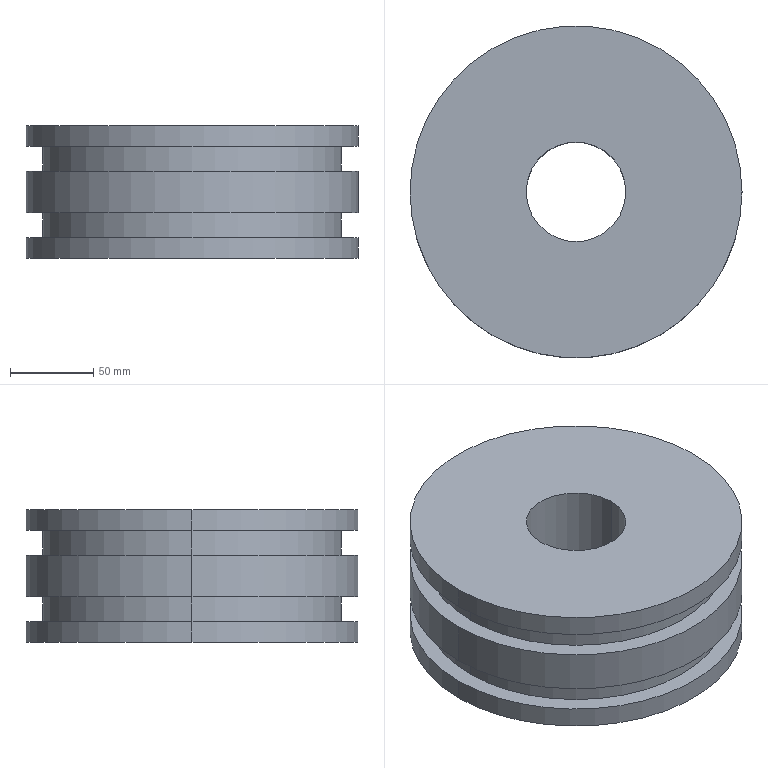Part | SolidWorks | features Extrusion 1, ICE 1, MirrorPattern 1 | 1 solid | 18 faces | box 200 x 200 x 80 mm | volume 2108009 mm3 | cylinder 12 | plane 6 | commonest cylinder face diameters 200 x6 180 x4 60 x2
STEP:
#1=CARTESIAN_POINT('',(90.,0.,-27.5));
#2=VERTEX_POINT('',#1);
#3=CARTESIAN_POINT('',(-90.,0.,-27.5));
#4=VERTEX_POINT('',#3);
#5=CARTESIAN_POINT('',(0.,0.,-27.5));
#6=DIRECTION('',(0.,0.,1.));
#7=DIRECTION('',(1.,0.,0.));
#8=AXIS2_PLACEMENT_3D('',#5,#6,#7);
#9=CIRCLE('',#8,90.);
#10=EDGE_CURVE('',#2,#4,#9,.T.);
#11=ORIENTED_EDGE('',*,*,#10,.T.);
#12=CARTESIAN_POINT('',(-90.,0.,-12.5));
#13=VERTEX_POINT('',#12);
#14=CARTESIAN_POINT('',(-90.,0.,-27.5));
#15=DIRECTION('',(0.,0.,1.));
#16=VECTOR('',#15,1000.);
#17=LINE('',#14,#16);
#18=EDGE_CURVE('',#4,#13,#17,.T.);
#19=ORIENTED_EDGE('',*,*,#18,.T.);
#20=CARTESIAN_POINT('',(90.,0.,-12.5));
#21=VERTEX_POINT('',#20);
#22=CARTESIAN_POINT('',(0.,0.,-12.5));
#23=DIRECTION('',(0.,0.,1.));
#24=DIRECTION('',(1.,0.,0.));
#25=AXIS2_PLACEMENT_3D('',#22,#23,#24);
#26=CIRCLE('',#25,90.);
#27=EDGE_CURVE('',#21,#13,#26,.T.);
#28=ORIENTED_EDGE('',*,*,#27,.F.);
#29=CARTESIAN_POINT('',(90.,0.,-27.5));
#30=DIRECTION('',(0.,0.,1.));
#31=VECTOR('',#30,1000.);
#32=LINE('',#29,#31);
#33=EDGE_CURVE('',#2,#21,#32,.T.);
#34=ORIENTED_EDGE('',*,*,#33,.F.);
#35=EDGE_LOOP('',(#11,#19,#28,#34));
#36=FACE_OUTER_BOUND('',#35,.T.);
#37=CARTESIAN_POINT('',(0.,0.,-27.5));
#38=DIRECTION('',(0.,0.,1.));
#39=DIRECTION('',(1.,0.,0.));
#40=AXIS2_PLACEMENT_3D('',#37,#38,#39);
#41=CYLINDRICAL_SURFACE('',#40,90.);
#42=ADVANCED_FACE('',(#36),#41,.T.);
#43=CARTESIAN_POINT('',(90.,0.,27.5));
#44=VERTEX_POINT('',#43);
#45=CARTESIAN_POINT('',(-90.,0.,27.5));
#46=VERTEX_POINT('',#45);
#47=CARTESIAN_POINT('',(0.,0.,27.5));
#48=DIRECTION('',(0.,0.,1.));
#49=DIRECTION('',(1.,0.,0.));
#50=AXIS2_PLACEMENT_3D('',#47,#48,#49);
#51=CIRCLE('',#50,90.);
#52=EDGE_CURVE('',#44,#46,#51,.T.);
#53=ORIENTED_EDGE('',*,*,#52,.F.);
#54=CARTESIAN_POINT('',(90.,0.,12.5));
#55=VERTEX_POINT('',#54);
#56=CARTESIAN_POINT('',(90.,0.,27.5));
#57=DIRECTION('',(0.,0.,-1.));
#58=VECTOR('',#57,1000.);
#59=LINE('',#56,#58);
#60=EDGE_CURVE('',#44,#55,#59,.T.);
#61=ORIENTED_EDGE('',*,*,#60,.T.);
#62=CARTESIAN_POINT('',(-90.,0.,12.5));
#63=VERTEX_POINT('',#62);
#64=CARTESIAN_POINT('',(0.,0.,12.5));
#65=DIRECTION('',(0.,0.,1.));
#66=DIRECTION('',(1.,0.,0.));
#67=AXIS2_PLACEMENT_3D('',#64,#65,#66);
#68=CIRCLE('',#67,90.);
#69=EDGE_CURVE('',#55,#63,#68,.T.);
#70=ORIENTED_EDGE('',*,*,#69,.T.);
#71=CARTESIAN_POINT('',(-90.,0.,27.5));
#72=DIRECTION('',(0.,0.,-1.));
#73=VECTOR('',#72,1000.);
#74=LINE('',#71,#73);
#75=EDGE_CURVE('',#46,#63,#74,.T.);
#76=ORIENTED_EDGE('',*,*,#75,.F.);
#77=EDGE_LOOP('',(#53,#61,#70,#76));
#78=FACE_OUTER_BOUND('',#77,.T.);
#79=CARTESIAN_POINT('',(0.,0.,27.5));
#80=DIRECTION('',(0.,0.,-1.));
#81=DIRECTION('',(-1.,0.,0.));
#82=AXIS2_PLACEMENT_3D('',#79,#80,#81);
#83=CYLINDRICAL_SURFACE('',#82,90.);
#84=ADVANCED_FACE('',(#78),#83,.T.);
#85=CARTESIAN_POINT('',(-30.,0.,40.));
#86=VERTEX_POINT('',#85);
#87=CARTESIAN_POINT('',(30.,0.,40.));
#88=VERTEX_POINT('',#87);
#89=CARTESIAN_POINT('',(0.,0.,40.));
#90=DIRECTION('',(0.,0.,1.));
#91=DIRECTION('',(1.,0.,0.));
#92=AXIS2_PLACEMENT_3D('',#89,#90,#91);
#93=CIRCLE('',#92,30.);
#94=EDGE_CURVE('',#86,#88,#93,.T.);
#95=ORIENTED_EDGE('',*,*,#94,.T.);
#96=CARTESIAN_POINT('',(30.,0.,-40.));
#97=VERTEX_POINT('',#96);
#98=CARTESIAN_POINT('',(30.,0.,40.));
#99=DIRECTION('',(0.,0.,-1.));
#100=VECTOR('',#99,1000.);
#101=LINE('',#98,#100);
#102=EDGE_CURVE('',#88,#97,#101,.T.);
#103=ORIENTED_EDGE('',*,*,#102,.T.);
#104=CARTESIAN_POINT('',(-30.,0.,-40.));
#105=VERTEX_POINT('',#104);
#106=CARTESIAN_POINT('',(0.,0.,-40.));
#107=DIRECTION('',(0.,0.,1.));
#108=DIRECTION('',(1.,0.,0.));
#109=AXIS2_PLACEMENT_3D('',#106,#107,#108);
#110=CIRCLE('',#109,30.);
#111=EDGE_CURVE('',#105,#97,#110,.T.);
#112=ORIENTED_EDGE('',*,*,#111,.F.);
#113=CARTESIAN_POINT('',(-30.,0.,40.));
#114=DIRECTION('',(0.,0.,-1.));
#115=VECTOR('',#114,1000.);
#116=LINE('',#113,#115);
#117=EDGE_CURVE('',#86,#105,#116,.T.);
#118=ORIENTED_EDGE('',*,*,#117,.F.);
#119=EDGE_LOOP('',(#95,#103,#112,#118));
#120=FACE_OUTER_BOUND('',#119,.T.);
#121=CARTESIAN_POINT('',(0.,0.,40.));
#122=DIRECTION('',(0.,0.,-1.));
#123=DIRECTION('',(-1.,0.,0.));
#124=AXIS2_PLACEMENT_3D('',#121,#122,#123);
#125=CYLINDRICAL_SURFACE('',#124,30.);
#126=ADVANCED_FACE('',(#120),#125,.F.);
#127=CARTESIAN_POINT('',(100.,0.,40.));
#128=VERTEX_POINT('',#127);
#129=CARTESIAN_POINT('',(-100.,0.,40.));
#130=VERTEX_POINT('',#129);
#131=CARTESIAN_POINT('',(0.,0.,40.));
#132=DIRECTION('',(0.,0.,1.));
#133=DIRECTION('',(1.,0.,0.));
#134=AXIS2_PLACEMENT_3D('',#131,#132,#133);
#135=CIRCLE('',#134,100.);
#136=EDGE_CURVE('',#128,#130,#135,.T.);
#137=ORIENTED_EDGE('',*,*,#136,.F.);
#138=CARTESIAN_POINT('',(100.,0.,27.5));
#139=VERTEX_POINT('',#138);
#140=CARTESIAN_POINT('',(100.,0.,40.));
#141=DIRECTION('',(0.,0.,-1.));
#142=VECTOR('',#141,1000.);
#143=LINE('',#140,#142);
#144=EDGE_CURVE('',#128,#139,#143,.T.);
#145=ORIENTED_EDGE('',*,*,#144,.T.);
#146=CARTESIAN_POINT('',(-100.,0.,27.5));
#147=VERTEX_POINT('',#146);
#148=CARTESIAN_POINT('',(0.,0.,27.5));
#149=DIRECTION('',(0.,0.,1.));
#150=DIRECTION('',(1.,0.,0.));
#151=AXIS2_PLACEMENT_3D('',#148,#149,#150);
#152=CIRCLE('',#151,100.);
#153=EDGE_CURVE('',#139,#147,#152,.T.);
#154=ORIENTED_EDGE('',*,*,#153,.T.);
#155=CARTESIAN_POINT('',(-100.,0.,40.));
#156=DIRECTION('',(0.,0.,-1.));
#157=VECTOR('',#156,1000.);
#158=LINE('',#155,#157);
#159=EDGE_CURVE('',#130,#147,#158,.T.);
#160=ORIENTED_EDGE('',*,*,#159,.F.);
#161=EDGE_LOOP('',(#137,#145,#154,#160));
#162=FACE_OUTER_BOUND('',#161,.T.);
#163=CARTESIAN_POINT('',(0.,0.,40.));
#164=DIRECTION('',(0.,0.,-1.));
#165=DIRECTION('',(-1.,0.,0.));
#166=AXIS2_PLACEMENT_3D('',#163,#164,#165);
#167=CYLINDRICAL_SURFACE('',#166,100.);
#168=ADVANCED_FACE('',(#162),#167,.T.);
#169=CARTESIAN_POINT('',(100.,0.,-27.5));
#170=VERTEX_POINT('',#169);
#171=CARTESIAN_POINT('',(-100.,0.,-27.5));
#172=VERTEX_POINT('',#171);
#173=CARTESIAN_POINT('',(0.,0.,-27.5));
#174=DIRECTION('',(0.,0.,1.));
#175=DIRECTION('',(1.,0.,0.));
#176=AXIS2_PLACEMENT_3D('',#173,#174,#175);
#177=CIRCLE('',#176,100.);
#178=EDGE_CURVE('',#170,#172,#177,.T.);
#179=ORIENTED_EDGE('',*,*,#178,.F.);
#180=CARTESIAN_POINT('',(100.,0.,-40.));
#181=VERTEX_POINT('',#180);
#182=CARTESIAN_POINT('',(100.,0.,40.));
#183=DIRECTION('',(0.,0.,-1.));
#184=VECTOR('',#183,1000.);
#185=LINE('',#182,#184);
#186=EDGE_CURVE('',#170,#181,#185,.T.);
#187=ORIENTED_EDGE('',*,*,#186,.T.);
#188=CARTESIAN_POINT('',(-100.,0.,-40.));
#189=VERTEX_POINT('',#188);
#190=CARTESIAN_POINT('',(0.,0.,-40.));
#191=DIRECTION('',(0.,0.,1.));
#192=DIRECTION('',(1.,0.,0.));
#193=AXIS2_PLACEMENT_3D('',#190,#191,#192);
#194=CIRCLE('',#193,100.);
#195=EDGE_CURVE('',#181,#189,#194,.T.);
#196=ORIENTED_EDGE('',*,*,#195,.T.);
#197=CARTESIAN_POINT('',(-100.,0.,40.));
#198=DIRECTION('',(0.,0.,-1.));
#199=VECTOR('',#198,1000.);
#200=LINE('',#197,#199);
#201=EDGE_CURVE('',#172,#189,#200,.T.);
#202=ORIENTED_EDGE('',*,*,#201,.F.);
#203=EDGE_LOOP('',(#179,#187,#196,#202));
#204=FACE_OUTER_BOUND('',#203,.T.);
#205=CARTESIAN_POINT('',(0.,0.,40.));
#206=DIRECTION('',(0.,0.,-1.));
#207=DIRECTION('',(-1.,0.,0.));
#208=AXIS2_PLACEMENT_3D('',#205,#206,#207);
#209=CYLINDRICAL_SURFACE('',#208,100.);
#210=ADVANCED_FACE('',(#204),#209,.T.);
#211=CARTESIAN_POINT('',(100.,0.,12.5));
#212=VERTEX_POINT('',#211);
#213=CARTESIAN_POINT('',(-100.,0.,12.5));
#214=VERTEX_POINT('',#213);
#215=CARTESIAN_POINT('',(0.,0.,12.5));
#216=DIRECTION('',(0.,0.,1.));
#217=DIRECTION('',(1.,0.,0.));
#218=AXIS2_PLACEMENT_3D('',#215,#216,#217);
#219=CIRCLE('',#218,100.);
#220=EDGE_CURVE('',#212,#214,#219,.T.);
#221=ORIENTED_EDGE('',*,*,#220,.F.);
#222=CARTESIAN_POINT('',(100.,0.,-12.5));
#223=VERTEX_POINT('',#222);
#224=CARTESIAN_POINT('',(100.,0.,40.));
#225=DIRECTION('',(0.,0.,-1.));
#226=VECTOR('',#225,1000.);
#227=LINE('',#224,#226);
#228=EDGE_CURVE('',#212,#223,#227,.T.);
#229=ORIENTED_EDGE('',*,*,#228,.T.);
#230=CARTESIAN_POINT('',(-100.,0.,-12.5));
#231=VERTEX_POINT('',#230);
#232=CARTESIAN_POINT('',(0.,0.,-12.5));
#233=DIRECTION('',(0.,0.,1.));
#234=DIRECTION('',(1.,0.,0.));
#235=AXIS2_PLACEMENT_3D('',#232,#233,#234);
#236=CIRCLE('',#235,100.);
#237=EDGE_CURVE('',#223,#231,#236,.T.);
#238=ORIENTED_EDGE('',*,*,#237,.T.);
#239=CARTESIAN_POINT('',(-100.,0.,40.));
#240=DIRECTION('',(0.,0.,-1.));
#241=VECTOR('',#240,1000.);
#242=LINE('',#239,#241);
#243=EDGE_CURVE('',#214,#231,#242,.T.);
#244=ORIENTED_EDGE('',*,*,#243,.F.);
#245=EDGE_LOOP('',(#221,#229,#238,#244));
#246=FACE_OUTER_BOUND('',#245,.T.);
#247=CARTESIAN_POINT('',(0.,0.,40.));
#248=DIRECTION('',(0.,0.,-1.));
#249=DIRECTION('',(-1.,0.,0.));
#250=AXIS2_PLACEMENT_3D('',#247,#248,#249);
#251=CYLINDRICAL_SURFACE('',#250,100.);
#252=ADVANCED_FACE('',(#246),#251,.T.);
#253=ORIENTED_EDGE('',*,*,#228,.F.);
#254=CARTESIAN_POINT('',(0.,0.,12.5));
#255=DIRECTION('',(0.,0.,1.));
#256=DIRECTION('',(1.,0.,0.));
#257=AXIS2_PLACEMENT_3D('',#254,#255,#256);
#258=CIRCLE('',#257,100.);
#259=EDGE_CURVE('',#214,#212,#258,.T.);
#260=ORIENTED_EDGE('',*,*,#259,.F.);
#261=ORIENTED_EDGE('',*,*,#243,.T.);
#262=CARTESIAN_POINT('',(0.,0.,-12.5));
#263=DIRECTION('',(0.,0.,1.));
#264=DIRECTION('',(1.,0.,0.));
#265=AXIS2_PLACEMENT_3D('',#262,#263,#264);
#266=CIRCLE('',#265,100.);
#267=EDGE_CURVE('',#231,#223,#266,.T.);
#268=ORIENTED_EDGE('',*,*,#267,.T.);
#269=EDGE_LOOP('',(#253,#260,#261,#268));
#270=FACE_OUTER_BOUND('',#269,.T.);
#271=CARTESIAN_POINT('',(0.,0.,40.));
#272=DIRECTION('',(0.,0.,-1.));
#273=DIRECTION('',(-1.,0.,0.));
#274=AXIS2_PLACEMENT_3D('',#271,#272,#273);
#275=CYLINDRICAL_SURFACE('',#274,100.);
#276=ADVANCED_FACE('',(#270),#275,.T.);
#277=ORIENTED_EDGE('',*,*,#186,.F.);
#278=CARTESIAN_POINT('',(0.,0.,-27.5));
#279=DIRECTION('',(0.,0.,1.));
#280=DIRECTION('',(1.,0.,0.));
#281=AXIS2_PLACEMENT_3D('',#278,#279,#280);
#282=CIRCLE('',#281,100.);
#283=EDGE_CURVE('',#172,#170,#282,.T.);
#284=ORIENTED_EDGE('',*,*,#283,.F.);
#285=ORIENTED_EDGE('',*,*,#201,.T.);
#286=CARTESIAN_POINT('',(0.,0.,-40.));
#287=DIRECTION('',(0.,0.,1.));
#288=DIRECTION('',(1.,0.,0.));
#289=AXIS2_PLACEMENT_3D('',#286,#287,#288);
#290=CIRCLE('',#289,100.);
#291=EDGE_CURVE('',#189,#181,#290,.T.);
#292=ORIENTED_EDGE('',*,*,#291,.T.);
#293=EDGE_LOOP('',(#277,#284,#285,#292));
#294=FACE_OUTER_BOUND('',#293,.T.);
#295=CARTESIAN_POINT('',(0.,0.,40.));
#296=DIRECTION('',(0.,0.,-1.));
#297=DIRECTION('',(-1.,0.,0.));
#298=AXIS2_PLACEMENT_3D('',#295,#296,#297);
#299=CYLINDRICAL_SURFACE('',#298,100.);
#300=ADVANCED_FACE('',(#294),#299,.T.);
#301=CARTESIAN_POINT('',(0.,0.,40.));
#302=DIRECTION('',(0.,0.,1.));
#303=DIRECTION('',(1.,0.,0.));
#304=AXIS2_PLACEMENT_3D('',#301,#302,#303);
#305=CIRCLE('',#304,100.);
#306=EDGE_CURVE('',#130,#128,#305,.T.);
#307=ORIENTED_EDGE('',*,*,#306,.T.);
#308=ORIENTED_EDGE('',*,*,#136,.T.);
#309=EDGE_LOOP('',(#307,#308));
#310=FACE_OUTER_BOUND('',#309,.T.);
#311=ORIENTED_EDGE('',*,*,#94,.F.);
#312=CARTESIAN_POINT('',(0.,0.,40.));
#313=DIRECTION('',(0.,0.,1.));
#314=DIRECTION('',(1.,0.,0.));
#315=AXIS2_PLACEMENT_3D('',#312,#313,#314);
#316=CIRCLE('',#315,30.);
#317=EDGE_CURVE('',#88,#86,#316,.T.);
#318=ORIENTED_EDGE('',*,*,#317,.F.);
#319=EDGE_LOOP('',(#311,#318));
#320=FACE_BOUND('',#319,.T.);
#321=CARTESIAN_POINT('',(0.,0.,40.));
#322=DIRECTION('',(0.,0.,1.));
#323=DIRECTION('',(1.,0.,0.));
#324=AXIS2_PLACEMENT_3D('',#321,#322,#323);
#325=PLANE('',#324);
#326=ADVANCED_FACE('',(#310,#320),#325,.T.);
#327=ORIENTED_EDGE('',*,*,#291,.F.);
#328=ORIENTED_EDGE('',*,*,#195,.F.);
#329=EDGE_LOOP('',(#327,#328));
#330=FACE_OUTER_BOUND('',#329,.T.);
#331=ORIENTED_EDGE('',*,*,#111,.T.);
#332=CARTESIAN_POINT('',(0.,0.,-40.));
#333=DIRECTION('',(0.,0.,1.));
#334=DIRECTION('',(1.,0.,0.));
#335=AXIS2_PLACEMENT_3D('',#332,#333,#334);
#336=CIRCLE('',#335,30.);
#337=EDGE_CURVE('',#97,#105,#336,.T.);
#338=ORIENTED_EDGE('',*,*,#337,.T.);
#339=EDGE_LOOP('',(#331,#338));
#340=FACE_BOUND('',#339,.T.);
#341=CARTESIAN_POINT('',(0.,0.,-40.));
#342=DIRECTION('',(0.,0.,1.));
#343=DIRECTION('',(1.,0.,0.));
#344=AXIS2_PLACEMENT_3D('',#341,#342,#343);
#345=PLANE('',#344);
#346=ADVANCED_FACE('',(#330,#340),#345,.F.);
#347=ORIENTED_EDGE('',*,*,#144,.F.);
#348=ORIENTED_EDGE('',*,*,#306,.F.);
#349=ORIENTED_EDGE('',*,*,#159,.T.);
#350=CARTESIAN_POINT('',(0.,0.,27.5));
#351=DIRECTION('',(0.,0.,1.));
#352=DIRECTION('',(1.,0.,0.));
#353=AXIS2_PLACEMENT_3D('',#350,#351,#352);
#354=CIRCLE('',#353,100.);
#355=EDGE_CURVE('',#147,#139,#354,.T.);
#356=ORIENTED_EDGE('',*,*,#355,.T.);
#357=EDGE_LOOP('',(#347,#348,#349,#356));
#358=FACE_OUTER_BOUND('',#357,.T.);
#359=CARTESIAN_POINT('',(0.,0.,40.));
#360=DIRECTION('',(0.,0.,-1.));
#361=DIRECTION('',(-1.,0.,0.));
#362=AXIS2_PLACEMENT_3D('',#359,#360,#361);
#363=CYLINDRICAL_SURFACE('',#362,100.);
#364=ADVANCED_FACE('',(#358),#363,.T.);
#365=ORIENTED_EDGE('',*,*,#102,.F.);
#366=ORIENTED_EDGE('',*,*,#317,.T.);
#367=ORIENTED_EDGE('',*,*,#117,.T.);
#368=ORIENTED_EDGE('',*,*,#337,.F.);
#369=EDGE_LOOP('',(#365,#366,#367,#368));
#370=FACE_OUTER_BOUND('',#369,.T.);
#371=CARTESIAN_POINT('',(0.,0.,40.));
#372=DIRECTION('',(0.,0.,-1.));
#373=DIRECTION('',(-1.,0.,0.));
#374=AXIS2_PLACEMENT_3D('',#371,#372,#373);
#375=CYLINDRICAL_SURFACE('',#374,30.);
#376=ADVANCED_FACE('',(#370),#375,.F.);
#377=ORIENTED_EDGE('',*,*,#355,.F.);
#378=ORIENTED_EDGE('',*,*,#153,.F.);
#379=EDGE_LOOP('',(#377,#378));
#380=FACE_OUTER_BOUND('',#379,.T.);
#381=CARTESIAN_POINT('',(0.,0.,27.5));
#382=DIRECTION('',(0.,0.,1.));
#383=DIRECTION('',(1.,0.,0.));
#384=AXIS2_PLACEMENT_3D('',#381,#382,#383);
#385=CIRCLE('',#384,90.);
#386=EDGE_CURVE('',#46,#44,#385,.T.);
#387=ORIENTED_EDGE('',*,*,#386,.T.);
#388=ORIENTED_EDGE('',*,*,#52,.T.);
#389=EDGE_LOOP('',(#387,#388));
#390=FACE_BOUND('',#389,.T.);
#391=CARTESIAN_POINT('',(0.,0.,27.5));
#392=DIRECTION('',(0.,0.,1.));
#393=DIRECTION('',(1.,0.,0.));
#394=AXIS2_PLACEMENT_3D('',#391,#392,#393);
#395=PLANE('',#394);
#396=ADVANCED_FACE('',(#380,#390),#395,.F.);
#397=ORIENTED_EDGE('',*,*,#259,.T.);
#398=ORIENTED_EDGE('',*,*,#220,.T.);
#399=EDGE_LOOP('',(#397,#398));
#400=FACE_OUTER_BOUND('',#399,.T.);
#401=CARTESIAN_POINT('',(0.,0.,12.5));
#402=DIRECTION('',(0.,0.,1.));
#403=DIRECTION('',(1.,0.,0.));
#404=AXIS2_PLACEMENT_3D('',#401,#402,#403);
#405=CIRCLE('',#404,90.);
#406=EDGE_CURVE('',#63,#55,#405,.T.);
#407=ORIENTED_EDGE('',*,*,#406,.F.);
#408=ORIENTED_EDGE('',*,*,#69,.F.);
#409=EDGE_LOOP('',(#407,#408));
#410=FACE_BOUND('',#409,.T.);
#411=CARTESIAN_POINT('',(0.,0.,12.5));
#412=DIRECTION('',(0.,0.,1.));
#413=DIRECTION('',(1.,0.,0.));
#414=AXIS2_PLACEMENT_3D('',#411,#412,#413);
#415=PLANE('',#414);
#416=ADVANCED_FACE('',(#400,#410),#415,.T.);
#417=ORIENTED_EDGE('',*,*,#60,.F.);
#418=ORIENTED_EDGE('',*,*,#386,.F.);
#419=ORIENTED_EDGE('',*,*,#75,.T.);
#420=ORIENTED_EDGE('',*,*,#406,.T.);
#421=EDGE_LOOP('',(#417,#418,#419,#420));
#422=FACE_OUTER_BOUND('',#421,.T.);
#423=CARTESIAN_POINT('',(0.,0.,27.5));
#424=DIRECTION('',(0.,0.,-1.));
#425=DIRECTION('',(-1.,0.,0.));
#426=AXIS2_PLACEMENT_3D('',#423,#424,#425);
#427=CYLINDRICAL_SURFACE('',#426,90.);
#428=ADVANCED_FACE('',(#422),#427,.T.);
#429=ORIENTED_EDGE('',*,*,#10,.F.);
#430=CARTESIAN_POINT('',(0.,0.,-27.5));
#431=DIRECTION('',(0.,0.,1.));
#432=DIRECTION('',(1.,0.,0.));
#433=AXIS2_PLACEMENT_3D('',#430,#431,#432);
#434=CIRCLE('',#433,90.);
#435=EDGE_CURVE('',#4,#2,#434,.T.);
#436=ORIENTED_EDGE('',*,*,#435,.F.);
#437=EDGE_LOOP('',(#429,#436));
#438=FACE_BOUND('',#437,.T.);
#439=ORIENTED_EDGE('',*,*,#283,.T.);
#440=ORIENTED_EDGE('',*,*,#178,.T.);
#441=EDGE_LOOP('',(#439,#440));
#442=FACE_OUTER_BOUND('',#441,.T.);
#443=CARTESIAN_POINT('',(0.,0.,-27.5));
#444=DIRECTION('',(0.,0.,-1.));
#445=DIRECTION('',(1.,0.,0.));
#446=AXIS2_PLACEMENT_3D('',#443,#444,#445);
#447=PLANE('',#446);
#448=ADVANCED_FACE('',(#438,#442),#447,.F.);
#449=ORIENTED_EDGE('',*,*,#27,.T.);
#450=CARTESIAN_POINT('',(0.,0.,-12.5));
#451=DIRECTION('',(0.,0.,1.));
#452=DIRECTION('',(1.,0.,0.));
#453=AXIS2_PLACEMENT_3D('',#450,#451,#452);
#454=CIRCLE('',#453,90.);
#455=EDGE_CURVE('',#13,#21,#454,.T.);
#456=ORIENTED_EDGE('',*,*,#455,.T.);
#457=EDGE_LOOP('',(#449,#456));
#458=FACE_BOUND('',#457,.T.);
#459=ORIENTED_EDGE('',*,*,#267,.F.);
#460=ORIENTED_EDGE('',*,*,#237,.F.);
#461=EDGE_LOOP('',(#459,#460));
#462=FACE_OUTER_BOUND('',#461,.T.);
#463=CARTESIAN_POINT('',(0.,0.,-12.5));
#464=DIRECTION('',(0.,0.,-1.));
#465=DIRECTION('',(1.,0.,0.));
#466=AXIS2_PLACEMENT_3D('',#463,#464,#465);
#467=PLANE('',#466);
#468=ADVANCED_FACE('',(#458,#462),#467,.T.);
#469=ORIENTED_EDGE('',*,*,#18,.F.);
#470=ORIENTED_EDGE('',*,*,#435,.T.);
#471=ORIENTED_EDGE('',*,*,#33,.T.);
#472=ORIENTED_EDGE('',*,*,#455,.F.);
#473=EDGE_LOOP('',(#469,#470,#471,#472));
#474=FACE_OUTER_BOUND('',#473,.T.);
#475=CARTESIAN_POINT('',(0.,0.,-27.5));
#476=DIRECTION('',(0.,0.,1.));
#477=DIRECTION('',(1.,0.,0.));
#478=AXIS2_PLACEMENT_3D('',#475,#476,#477);
#479=CYLINDRICAL_SURFACE('',#478,90.);
#480=ADVANCED_FACE('',(#474),#479,.T.);
#481=CLOSED_SHELL('',(#42,#84,#126,#168,#210,#252,#276,#300,#326,#346,#364,#376,#396,#416,#428,#448,#468,#480));
#482=MANIFOLD_SOLID_BREP('',#481);
#483=CARTESIAN_POINT('',(0.,0.,0.));
#484=DIRECTION('',(0.,0.,1.));
#485=DIRECTION('',(1.,0.,0.));
#486=AXIS2_PLACEMENT_3D('',#483,#484,#485);
#487=(LENGTH_UNIT()NAMED_UNIT(*)SI_UNIT(.MILLI.,.METRE.));
#488=UNCERTAINTY_MEASURE_WITH_UNIT(LENGTH_MEASURE(0.00001),#487,'','');
#489=(NAMED_UNIT(*)PLANE_ANGLE_UNIT()SI_UNIT($,.RADIAN.));
#490=(NAMED_UNIT(*)SI_UNIT($,.STERADIAN.)SOLID_ANGLE_UNIT());
#491=(GEOMETRIC_REPRESENTATION_CONTEXT(3)GLOBAL_UNCERTAINTY_ASSIGNED_CONTEXT((#488))GLOBAL_UNIT_ASSIGNED_CONTEXT((#487,#489,#490))REPRESENTATION_CONTEXT('',''));
#492=ADVANCED_BREP_SHAPE_REPRESENTATION('',(#482,#486),#491);